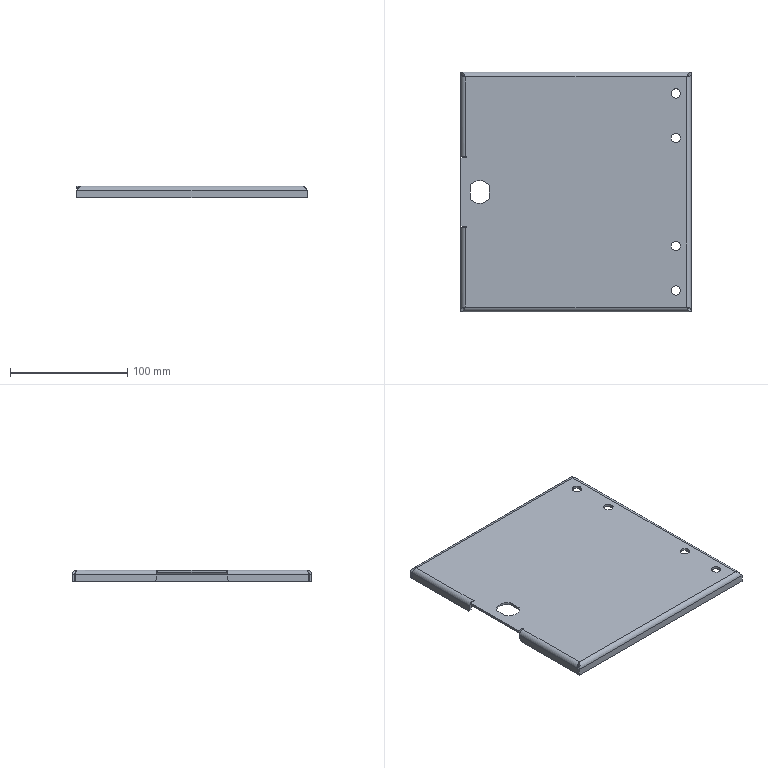Part | STEP file | SYL0380DJ1008_2_7_2_2-1_STEP | 1 solid | 68 faces | box 196 x 204 x 10 mm | volume 88727 mm3 | plane 40 | cylinder 20 | spline 8 | commonest cylinder face diameters 8 x13 4 x5 19.5 x2